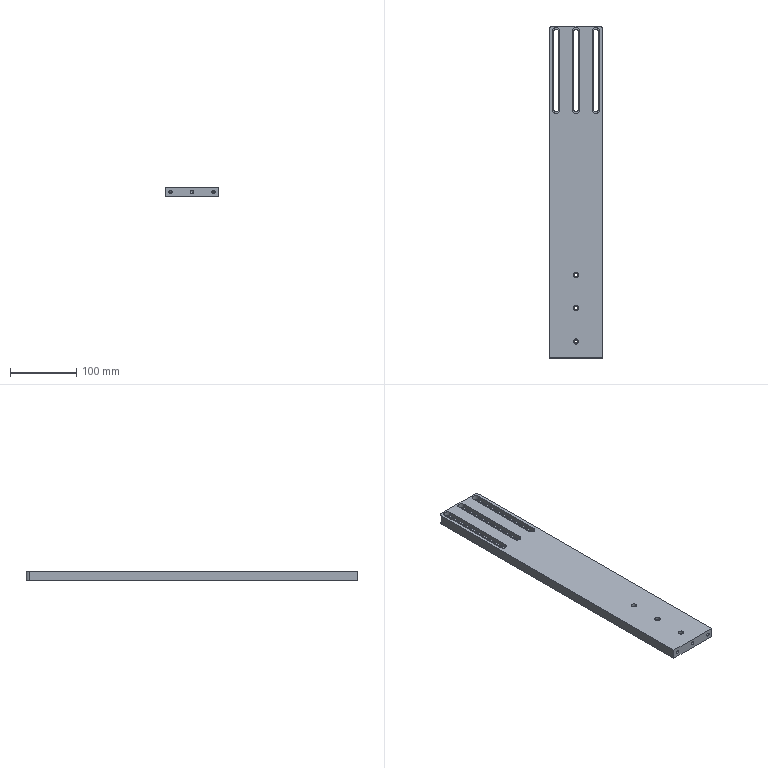Part | SolidWorks | features HoleWzd 4, Extrusion 1, Fillet 1, MirrorPattern 1 | 1 solid | 62 faces | box 80 x 500 x 15 mm | volume 549882 mm3 | cylinder 32 | plane 24 | cone 6 | commonest cylinder face diameters 4.5 x6 5 x6 6.6 x6 8 x6 11 x6 10 x2